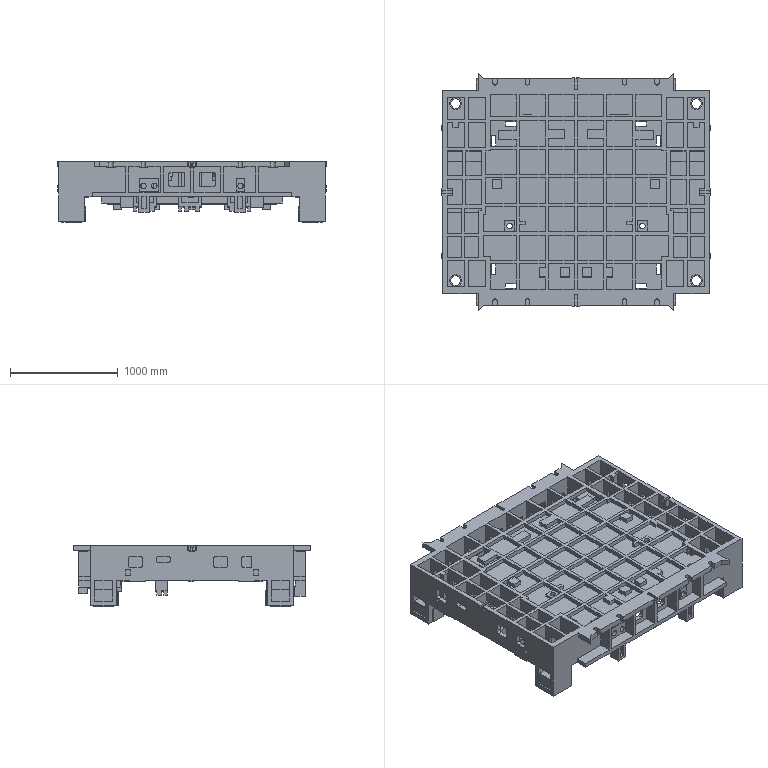Part | NX | features solid 2 | 1 solid | 1826 faces | box 2490 x 2200 x 565 mm | volume 558427884 mm3 | plane 1544 | cylinder 273 | cone 9 | commonest cylinder face diameters 40 x204 30 x26 10 x11 52 x8 80 x8 90 x4